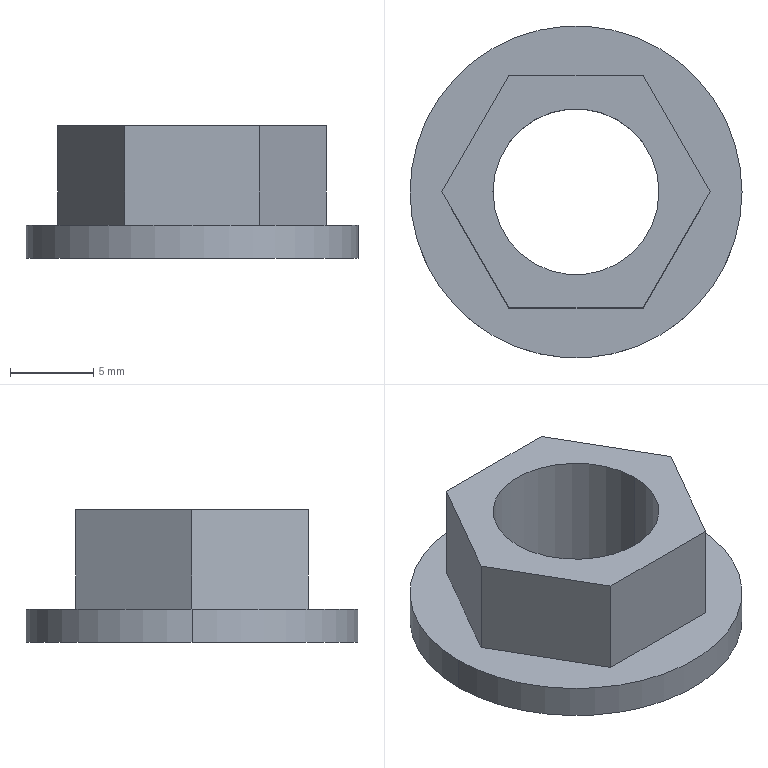Part | SolidWorks | features BaseBody 1 | 1 solid | 13 faces | box 20 x 20 x 8 mm | volume 1018 mm3 | plane 9 | cylinder 4 | commonest cylinder face diameters 10 x2 20 x2
STEP:
#1=CARTESIAN_POINT('',(5.,0.,0.));
#2=VERTEX_POINT('',#1);
#3=CARTESIAN_POINT('',(-5.,0.,0.));
#4=VERTEX_POINT('',#3);
#5=CARTESIAN_POINT('',(0.,0.,0.));
#6=DIRECTION('',(0.,0.,1.));
#7=DIRECTION('',(-1.,0.,0.));
#8=AXIS2_PLACEMENT_3D('',#5,#6,#7);
#9=CIRCLE('',#8,5.);
#10=EDGE_CURVE('',#2,#4,#9,.T.);
#11=ORIENTED_EDGE('',*,*,#10,.F.);
#12=CARTESIAN_POINT('',(5.,0.,8.));
#13=VERTEX_POINT('',#12);
#14=CARTESIAN_POINT('',(5.,0.,8.));
#15=DIRECTION('',(0.,0.,1.));
#16=VECTOR('',#15,1000.);
#17=LINE('',#14,#16);
#18=EDGE_CURVE('',#2,#13,#17,.T.);
#19=ORIENTED_EDGE('',*,*,#18,.T.);
#20=CARTESIAN_POINT('',(-5.,0.,8.));
#21=VERTEX_POINT('',#20);
#22=CARTESIAN_POINT('',(0.,0.,8.));
#23=DIRECTION('',(0.,0.,-1.));
#24=DIRECTION('',(-1.,0.,0.));
#25=AXIS2_PLACEMENT_3D('',#22,#23,#24);
#26=CIRCLE('',#25,5.);
#27=EDGE_CURVE('',#21,#13,#26,.T.);
#28=ORIENTED_EDGE('',*,*,#27,.F.);
#29=CARTESIAN_POINT('',(-5.,0.,8.));
#30=DIRECTION('',(0.,0.,1.));
#31=VECTOR('',#30,1000.);
#32=LINE('',#29,#31);
#33=EDGE_CURVE('',#4,#21,#32,.T.);
#34=ORIENTED_EDGE('',*,*,#33,.F.);
#35=EDGE_LOOP('',(#11,#19,#28,#34));
#36=FACE_OUTER_BOUND('',#35,.T.);
#37=CARTESIAN_POINT('',(0.,0.,8.));
#38=DIRECTION('',(0.,0.,1.));
#39=DIRECTION('',(-1.,0.,0.));
#40=AXIS2_PLACEMENT_3D('',#37,#38,#39);
#41=CYLINDRICAL_SURFACE('',#40,5.);
#42=ADVANCED_FACE('',(#36),#41,.F.);
#43=CARTESIAN_POINT('',(10.,0.,2.));
#44=VERTEX_POINT('',#43);
#45=CARTESIAN_POINT('',(-10.,0.,2.));
#46=VERTEX_POINT('',#45);
#47=CARTESIAN_POINT('',(0.,0.,2.));
#48=DIRECTION('',(0.,0.,1.));
#49=DIRECTION('',(-1.,0.,0.));
#50=AXIS2_PLACEMENT_3D('',#47,#48,#49);
#51=CIRCLE('',#50,10.);
#52=EDGE_CURVE('',#44,#46,#51,.T.);
#53=ORIENTED_EDGE('',*,*,#52,.F.);
#54=CARTESIAN_POINT('',(10.,0.,0.));
#55=VERTEX_POINT('',#54);
#56=CARTESIAN_POINT('',(10.,0.,0.));
#57=DIRECTION('',(0.,0.,-1.));
#58=VECTOR('',#57,1000.);
#59=LINE('',#56,#58);
#60=EDGE_CURVE('',#44,#55,#59,.T.);
#61=ORIENTED_EDGE('',*,*,#60,.T.);
#62=CARTESIAN_POINT('',(-10.,0.,0.));
#63=VERTEX_POINT('',#62);
#64=CARTESIAN_POINT('',(0.,0.,0.));
#65=DIRECTION('',(0.,0.,-1.));
#66=DIRECTION('',(-1.,0.,0.));
#67=AXIS2_PLACEMENT_3D('',#64,#65,#66);
#68=CIRCLE('',#67,10.);
#69=EDGE_CURVE('',#63,#55,#68,.T.);
#70=ORIENTED_EDGE('',*,*,#69,.F.);
#71=CARTESIAN_POINT('',(-10.,0.,0.));
#72=DIRECTION('',(0.,0.,-1.));
#73=VECTOR('',#72,1000.);
#74=LINE('',#71,#73);
#75=EDGE_CURVE('',#46,#63,#74,.T.);
#76=ORIENTED_EDGE('',*,*,#75,.F.);
#77=EDGE_LOOP('',(#53,#61,#70,#76));
#78=FACE_OUTER_BOUND('',#77,.T.);
#79=CARTESIAN_POINT('',(0.,0.,0.));
#80=DIRECTION('',(0.,0.,-1.));
#81=DIRECTION('',(-1.,0.,0.));
#82=AXIS2_PLACEMENT_3D('',#79,#80,#81);
#83=CYLINDRICAL_SURFACE('',#82,10.);
#84=ADVANCED_FACE('',(#78),#83,.T.);
#85=CARTESIAN_POINT('',(-4.041,-7.,2.));
#86=VERTEX_POINT('',#85);
#87=CARTESIAN_POINT('',(-8.083,0.,2.));
#88=VERTEX_POINT('',#87);
#89=CARTESIAN_POINT('',(-7.073,-1.75,2.));
#90=DIRECTION('',(-0.5,0.866,0.));
#91=VECTOR('',#90,1000.);
#92=LINE('',#89,#91);
#93=EDGE_CURVE('',#86,#88,#92,.T.);
#94=ORIENTED_EDGE('',*,*,#93,.F.);
#95=CARTESIAN_POINT('',(-4.041,-7.,8.));
#96=VERTEX_POINT('',#95);
#97=CARTESIAN_POINT('',(-4.041,-7.,2.));
#98=DIRECTION('',(0.,0.,1.));
#99=VECTOR('',#98,1000.);
#100=LINE('',#97,#99);
#101=EDGE_CURVE('',#86,#96,#100,.T.);
#102=ORIENTED_EDGE('',*,*,#101,.T.);
#103=CARTESIAN_POINT('',(-8.083,0.,8.));
#104=VERTEX_POINT('',#103);
#105=CARTESIAN_POINT('',(-4.041,-7.,8.));
#106=DIRECTION('',(0.5,-0.866,0.));
#107=VECTOR('',#106,1000.);
#108=LINE('',#105,#107);
#109=EDGE_CURVE('',#104,#96,#108,.T.);
#110=ORIENTED_EDGE('',*,*,#109,.F.);
#111=CARTESIAN_POINT('',(-8.083,0.,2.));
#112=DIRECTION('',(0.,0.,1.));
#113=VECTOR('',#112,1000.);
#114=LINE('',#111,#113);
#115=EDGE_CURVE('',#88,#104,#114,.T.);
#116=ORIENTED_EDGE('',*,*,#115,.F.);
#117=EDGE_LOOP('',(#94,#102,#110,#116));
#118=FACE_OUTER_BOUND('',#117,.T.);
#119=CARTESIAN_POINT('',(-8.083,0.,2.));
#120=DIRECTION('',(-0.866,-0.5,0.));
#121=DIRECTION('',(-0.5,0.866,0.));
#122=AXIS2_PLACEMENT_3D('',#119,#120,#121);
#123=PLANE('',#122);
#124=ADVANCED_FACE('',(#118),#123,.T.);
#125=CARTESIAN_POINT('',(-4.041,7.,2.));
#126=VERTEX_POINT('',#125);
#127=CARTESIAN_POINT('',(-5.052,5.25,2.));
#128=DIRECTION('',(0.5,0.866,0.));
#129=VECTOR('',#128,1000.);
#130=LINE('',#127,#129);
#131=EDGE_CURVE('',#88,#126,#130,.T.);
#132=ORIENTED_EDGE('',*,*,#131,.F.);
#133=ORIENTED_EDGE('',*,*,#115,.T.);
#134=CARTESIAN_POINT('',(-4.041,7.,8.));
#135=VERTEX_POINT('',#134);
#136=CARTESIAN_POINT('',(-8.083,0.,8.));
#137=DIRECTION('',(-0.5,-0.866,0.));
#138=VECTOR('',#137,1000.);
#139=LINE('',#136,#138);
#140=EDGE_CURVE('',#135,#104,#139,.T.);
#141=ORIENTED_EDGE('',*,*,#140,.F.);
#142=CARTESIAN_POINT('',(-4.041,7.,2.));
#143=DIRECTION('',(0.,0.,1.));
#144=VECTOR('',#143,1000.);
#145=LINE('',#142,#144);
#146=EDGE_CURVE('',#126,#135,#145,.T.);
#147=ORIENTED_EDGE('',*,*,#146,.F.);
#148=EDGE_LOOP('',(#132,#133,#141,#147));
#149=FACE_OUTER_BOUND('',#148,.T.);
#150=CARTESIAN_POINT('',(-4.041,7.,2.));
#151=DIRECTION('',(-0.866,0.5,0.));
#152=DIRECTION('',(0.,0.,1.));
#153=AXIS2_PLACEMENT_3D('',#150,#151,#152);
#154=PLANE('',#153);
#155=ADVANCED_FACE('',(#149),#154,.T.);
#156=CARTESIAN_POINT('',(4.041,7.,2.));
#157=VERTEX_POINT('',#156);
#158=CARTESIAN_POINT('',(2.021,7.,2.));
#159=DIRECTION('',(1.,0.,0.));
#160=VECTOR('',#159,1000.);
#161=LINE('',#158,#160);
#162=EDGE_CURVE('',#126,#157,#161,.T.);
#163=ORIENTED_EDGE('',*,*,#162,.F.);
#164=ORIENTED_EDGE('',*,*,#146,.T.);
#165=CARTESIAN_POINT('',(4.041,7.,8.));
#166=VERTEX_POINT('',#165);
#167=CARTESIAN_POINT('',(-4.041,7.,8.));
#168=DIRECTION('',(-1.,0.,0.));
#169=VECTOR('',#168,1000.);
#170=LINE('',#167,#169);
#171=EDGE_CURVE('',#166,#135,#170,.T.);
#172=ORIENTED_EDGE('',*,*,#171,.F.);
#173=CARTESIAN_POINT('',(4.041,7.,2.));
#174=DIRECTION('',(0.,0.,1.));
#175=VECTOR('',#174,1000.);
#176=LINE('',#173,#175);
#177=EDGE_CURVE('',#157,#166,#176,.T.);
#178=ORIENTED_EDGE('',*,*,#177,.F.);
#179=EDGE_LOOP('',(#163,#164,#172,#178));
#180=FACE_OUTER_BOUND('',#179,.T.);
#181=CARTESIAN_POINT('',(4.041,7.,2.));
#182=DIRECTION('',(0.,1.,0.));
#183=DIRECTION('',(1.,0.,0.));
#184=AXIS2_PLACEMENT_3D('',#181,#182,#183);
#185=PLANE('',#184);
#186=ADVANCED_FACE('',(#180),#185,.T.);
#187=CARTESIAN_POINT('',(8.083,0.,2.));
#188=VERTEX_POINT('',#187);
#189=CARTESIAN_POINT('',(7.073,1.75,2.));
#190=DIRECTION('',(0.5,-0.866,0.));
#191=VECTOR('',#190,1000.);
#192=LINE('',#189,#191);
#193=EDGE_CURVE('',#157,#188,#192,.T.);
#194=ORIENTED_EDGE('',*,*,#193,.F.);
#195=ORIENTED_EDGE('',*,*,#177,.T.);
#196=CARTESIAN_POINT('',(8.083,0.,8.));
#197=VERTEX_POINT('',#196);
#198=CARTESIAN_POINT('',(4.041,7.,8.));
#199=DIRECTION('',(-0.5,0.866,0.));
#200=VECTOR('',#199,1000.);
#201=LINE('',#198,#200);
#202=EDGE_CURVE('',#197,#166,#201,.T.);
#203=ORIENTED_EDGE('',*,*,#202,.F.);
#204=CARTESIAN_POINT('',(8.083,0.,2.));
#205=DIRECTION('',(0.,0.,1.));
#206=VECTOR('',#205,1000.);
#207=LINE('',#204,#206);
#208=EDGE_CURVE('',#188,#197,#207,.T.);
#209=ORIENTED_EDGE('',*,*,#208,.F.);
#210=EDGE_LOOP('',(#194,#195,#203,#209));
#211=FACE_OUTER_BOUND('',#210,.T.);
#212=CARTESIAN_POINT('',(8.083,0.,2.));
#213=DIRECTION('',(0.866,0.5,0.));
#214=DIRECTION('',(0.,0.,-1.));
#215=AXIS2_PLACEMENT_3D('',#212,#213,#214);
#216=PLANE('',#215);
#217=ADVANCED_FACE('',(#211),#216,.T.);
#218=CARTESIAN_POINT('',(4.041,-7.,2.));
#219=VERTEX_POINT('',#218);
#220=CARTESIAN_POINT('',(5.052,-5.25,2.));
#221=DIRECTION('',(-0.5,-0.866,0.));
#222=VECTOR('',#221,1000.);
#223=LINE('',#220,#222);
#224=EDGE_CURVE('',#188,#219,#223,.T.);
#225=ORIENTED_EDGE('',*,*,#224,.F.);
#226=ORIENTED_EDGE('',*,*,#208,.T.);
#227=CARTESIAN_POINT('',(4.041,-7.,8.));
#228=VERTEX_POINT('',#227);
#229=CARTESIAN_POINT('',(8.083,0.,8.));
#230=DIRECTION('',(0.5,0.866,0.));
#231=VECTOR('',#230,1000.);
#232=LINE('',#229,#231);
#233=EDGE_CURVE('',#228,#197,#232,.T.);
#234=ORIENTED_EDGE('',*,*,#233,.F.);
#235=CARTESIAN_POINT('',(4.041,-7.,2.));
#236=DIRECTION('',(0.,0.,1.));
#237=VECTOR('',#236,1000.);
#238=LINE('',#235,#237);
#239=EDGE_CURVE('',#219,#228,#238,.T.);
#240=ORIENTED_EDGE('',*,*,#239,.F.);
#241=EDGE_LOOP('',(#225,#226,#234,#240));
#242=FACE_OUTER_BOUND('',#241,.T.);
#243=CARTESIAN_POINT('',(4.041,-7.,2.));
#244=DIRECTION('',(0.866,-0.5,0.));
#245=DIRECTION('',(0.,0.,-1.));
#246=AXIS2_PLACEMENT_3D('',#243,#244,#245);
#247=PLANE('',#246);
#248=ADVANCED_FACE('',(#242),#247,.T.);
#249=CARTESIAN_POINT('',(-2.021,-7.,2.));
#250=DIRECTION('',(-1.,0.,0.));
#251=VECTOR('',#250,1000.);
#252=LINE('',#249,#251);
#253=EDGE_CURVE('',#219,#86,#252,.T.);
#254=ORIENTED_EDGE('',*,*,#253,.F.);
#255=ORIENTED_EDGE('',*,*,#239,.T.);
#256=CARTESIAN_POINT('',(4.041,-7.,8.));
#257=DIRECTION('',(1.,0.,0.));
#258=VECTOR('',#257,1000.);
#259=LINE('',#256,#258);
#260=EDGE_CURVE('',#96,#228,#259,.T.);
#261=ORIENTED_EDGE('',*,*,#260,.F.);
#262=ORIENTED_EDGE('',*,*,#101,.F.);
#263=EDGE_LOOP('',(#254,#255,#261,#262));
#264=FACE_OUTER_BOUND('',#263,.T.);
#265=CARTESIAN_POINT('',(-4.041,-7.,2.));
#266=DIRECTION('',(0.,-1.,0.));
#267=DIRECTION('',(-1.,0.,0.));
#268=AXIS2_PLACEMENT_3D('',#265,#266,#267);
#269=PLANE('',#268);
#270=ADVANCED_FACE('',(#264),#269,.T.);
#271=ORIENTED_EDGE('',*,*,#27,.T.);
#272=CARTESIAN_POINT('',(0.,0.,8.));
#273=DIRECTION('',(0.,0.,-1.));
#274=DIRECTION('',(-1.,0.,0.));
#275=AXIS2_PLACEMENT_3D('',#272,#273,#274);
#276=CIRCLE('',#275,5.);
#277=EDGE_CURVE('',#13,#21,#276,.T.);
#278=ORIENTED_EDGE('',*,*,#277,.T.);
#279=EDGE_LOOP('',(#271,#278));
#280=FACE_BOUND('',#279,.T.);
#281=ORIENTED_EDGE('',*,*,#260,.T.);
#282=ORIENTED_EDGE('',*,*,#233,.T.);
#283=ORIENTED_EDGE('',*,*,#202,.T.);
#284=ORIENTED_EDGE('',*,*,#171,.T.);
#285=ORIENTED_EDGE('',*,*,#140,.T.);
#286=ORIENTED_EDGE('',*,*,#109,.T.);
#287=EDGE_LOOP('',(#281,#282,#283,#284,#285,#286));
#288=FACE_OUTER_BOUND('',#287,.T.);
#289=CARTESIAN_POINT('',(0.,0.,8.));
#290=DIRECTION('',(0.,0.,1.));
#291=DIRECTION('',(1.,0.,0.));
#292=AXIS2_PLACEMENT_3D('',#289,#290,#291);
#293=PLANE('',#292);
#294=ADVANCED_FACE('',(#280,#288),#293,.T.);
#295=CARTESIAN_POINT('',(0.,0.,0.));
#296=DIRECTION('',(0.,0.,1.));
#297=DIRECTION('',(-1.,0.,0.));
#298=AXIS2_PLACEMENT_3D('',#295,#296,#297);
#299=CIRCLE('',#298,5.);
#300=EDGE_CURVE('',#4,#2,#299,.T.);
#301=ORIENTED_EDGE('',*,*,#300,.T.);
#302=ORIENTED_EDGE('',*,*,#10,.T.);
#303=EDGE_LOOP('',(#301,#302));
#304=FACE_BOUND('',#303,.T.);
#305=ORIENTED_EDGE('',*,*,#69,.T.);
#306=CARTESIAN_POINT('',(0.,0.,0.));
#307=DIRECTION('',(0.,0.,-1.));
#308=DIRECTION('',(-1.,0.,0.));
#309=AXIS2_PLACEMENT_3D('',#306,#307,#308);
#310=CIRCLE('',#309,10.);
#311=EDGE_CURVE('',#55,#63,#310,.T.);
#312=ORIENTED_EDGE('',*,*,#311,.T.);
#313=EDGE_LOOP('',(#305,#312));
#314=FACE_OUTER_BOUND('',#313,.T.);
#315=CARTESIAN_POINT('',(0.,0.,0.));
#316=DIRECTION('',(0.,0.,1.));
#317=DIRECTION('',(1.,0.,0.));
#318=AXIS2_PLACEMENT_3D('',#315,#316,#317);
#319=PLANE('',#318);
#320=ADVANCED_FACE('',(#304,#314),#319,.F.);
#321=ORIENTED_EDGE('',*,*,#93,.T.);
#322=ORIENTED_EDGE('',*,*,#131,.T.);
#323=ORIENTED_EDGE('',*,*,#162,.T.);
#324=ORIENTED_EDGE('',*,*,#193,.T.);
#325=ORIENTED_EDGE('',*,*,#224,.T.);
#326=ORIENTED_EDGE('',*,*,#253,.T.);
#327=EDGE_LOOP('',(#321,#322,#323,#324,#325,#326));
#328=FACE_BOUND('',#327,.T.);
#329=CARTESIAN_POINT('',(0.,0.,2.));
#330=DIRECTION('',(0.,0.,1.));
#331=DIRECTION('',(-1.,0.,0.));
#332=AXIS2_PLACEMENT_3D('',#329,#330,#331);
#333=CIRCLE('',#332,10.);
#334=EDGE_CURVE('',#46,#44,#333,.T.);
#335=ORIENTED_EDGE('',*,*,#334,.T.);
#336=ORIENTED_EDGE('',*,*,#52,.T.);
#337=EDGE_LOOP('',(#335,#336));
#338=FACE_OUTER_BOUND('',#337,.T.);
#339=CARTESIAN_POINT('',(0.,0.,2.));
#340=DIRECTION('',(0.,0.,1.));
#341=DIRECTION('',(1.,0.,0.));
#342=AXIS2_PLACEMENT_3D('',#339,#340,#341);
#343=PLANE('',#342);
#344=ADVANCED_FACE('',(#328,#338),#343,.T.);
#345=ORIENTED_EDGE('',*,*,#60,.F.);
#346=ORIENTED_EDGE('',*,*,#334,.F.);
#347=ORIENTED_EDGE('',*,*,#75,.T.);
#348=ORIENTED_EDGE('',*,*,#311,.F.);
#349=EDGE_LOOP('',(#345,#346,#347,#348));
#350=FACE_OUTER_BOUND('',#349,.T.);
#351=CARTESIAN_POINT('',(0.,0.,0.));
#352=DIRECTION('',(0.,0.,-1.));
#353=DIRECTION('',(-1.,0.,0.));
#354=AXIS2_PLACEMENT_3D('',#351,#352,#353);
#355=CYLINDRICAL_SURFACE('',#354,10.);
#356=ADVANCED_FACE('',(#350),#355,.T.);
#357=ORIENTED_EDGE('',*,*,#18,.F.);
#358=ORIENTED_EDGE('',*,*,#300,.F.);
#359=ORIENTED_EDGE('',*,*,#33,.T.);
#360=ORIENTED_EDGE('',*,*,#277,.F.);
#361=EDGE_LOOP('',(#357,#358,#359,#360));
#362=FACE_OUTER_BOUND('',#361,.T.);
#363=CARTESIAN_POINT('',(0.,0.,8.));
#364=DIRECTION('',(0.,0.,1.));
#365=DIRECTION('',(-1.,0.,0.));
#366=AXIS2_PLACEMENT_3D('',#363,#364,#365);
#367=CYLINDRICAL_SURFACE('',#366,5.);
#368=ADVANCED_FACE('',(#362),#367,.F.);
#369=CLOSED_SHELL('',(#42,#84,#124,#155,#186,#217,#248,#270,#294,#320,#344,#356,#368));
#370=MANIFOLD_SOLID_BREP('',#369);
#371=CARTESIAN_POINT('',(0.,0.,0.));
#372=DIRECTION('',(0.,0.,1.));
#373=DIRECTION('',(1.,0.,0.));
#374=AXIS2_PLACEMENT_3D('',#371,#372,#373);
#375=(LENGTH_UNIT()NAMED_UNIT(*)SI_UNIT(.MILLI.,.METRE.));
#376=UNCERTAINTY_MEASURE_WITH_UNIT(LENGTH_MEASURE(0.00001),#375,'','');
#377=(NAMED_UNIT(*)PLANE_ANGLE_UNIT()SI_UNIT($,.RADIAN.));
#378=(NAMED_UNIT(*)SI_UNIT($,.STERADIAN.)SOLID_ANGLE_UNIT());
#379=(GEOMETRIC_REPRESENTATION_CONTEXT(3)GLOBAL_UNCERTAINTY_ASSIGNED_CONTEXT((#376))GLOBAL_UNIT_ASSIGNED_CONTEXT((#375,#377,#378))REPRESENTATION_CONTEXT('',''));
#380=ADVANCED_BREP_SHAPE_REPRESENTATION('',(#370,#374),#379);